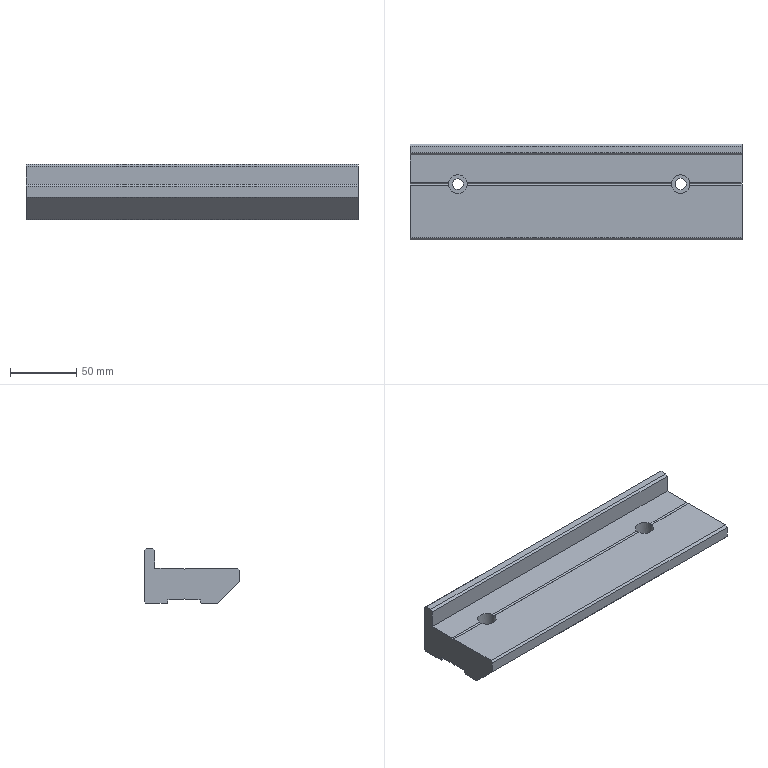Part | NX | features EXTRUDE 3, DATUM_CSYS 2, SKETCH 1 | 1 solid | 39 faces | box 250 x 72 x 41.5 mm | volume 446626 mm3 | plane 35 | cylinder 4 | commonest cylinder face diameters 14 x2 8 x1 8.5 x1
STEP:
#1=CARTESIAN_POINT('',(4843.54,6881.489,-37.5));
#2=VERTEX_POINT('',#1);
#3=CARTESIAN_POINT('',(4843.413,6882.489,-38.5));
#4=VERTEX_POINT('',#3);
#5=CARTESIAN_POINT('',(4839.54,6881.489,-37.5));
#6=DIRECTION('',(0.,-0.7071,-0.7071));
#7=DIRECTION('',(0.,-0.7071,0.7071));
#8=AXIS2_PLACEMENT_3D('',#5,#6,#7);
#9=ELLIPSE('',#8,5.657,4.);
#10=EDGE_CURVE('',#2,#4,#9,.F.);
#11=ORIENTED_EDGE('',*,*,#10,.F.);
#12=CARTESIAN_POINT('',(4843.413,6880.489,-38.5));
#13=VERTEX_POINT('',#12);
#14=CARTESIAN_POINT('',(4839.54,6881.489,-37.5));
#15=DIRECTION('',(0.,0.7071,-0.7071));
#16=DIRECTION('',(0.,0.7071,0.7071));
#17=AXIS2_PLACEMENT_3D('',#14,#15,#16);
#18=ELLIPSE('',#17,5.657,4.);
#19=EDGE_CURVE('',#13,#2,#18,.F.);
#20=ORIENTED_EDGE('',*,*,#19,.F.);
#21=CARTESIAN_POINT('',(4835.667,6880.489,-38.5));
#22=VERTEX_POINT('',#21);
#23=CARTESIAN_POINT('',(4839.54,6881.489,-38.5));
#24=DIRECTION('',(0.,0.,-1.));
#25=DIRECTION('',(-1.,0.,0.));
#26=AXIS2_PLACEMENT_3D('',#23,#24,#25);
#27=CIRCLE('',#26,4.);
#28=EDGE_CURVE('',#22,#13,#27,.F.);
#29=ORIENTED_EDGE('',*,*,#28,.F.);
#30=CARTESIAN_POINT('',(4835.54,6881.489,-37.5));
#31=VERTEX_POINT('',#30);
#32=CARTESIAN_POINT('',(4839.54,6881.489,-37.5));
#33=DIRECTION('',(0.,0.7071,-0.7071));
#34=DIRECTION('',(0.,0.7071,0.7071));
#35=AXIS2_PLACEMENT_3D('',#32,#33,#34);
#36=ELLIPSE('',#35,5.657,4.);
#37=EDGE_CURVE('',#31,#22,#36,.F.);
#38=ORIENTED_EDGE('',*,*,#37,.F.);
#39=CARTESIAN_POINT('',(4835.667,6882.489,-38.5));
#40=VERTEX_POINT('',#39);
#41=CARTESIAN_POINT('',(4839.54,6881.489,-37.5));
#42=DIRECTION('',(0.,-0.7071,-0.7071));
#43=DIRECTION('',(0.,-0.7071,0.7071));
#44=AXIS2_PLACEMENT_3D('',#41,#42,#43);
#45=ELLIPSE('',#44,5.657,4.);
#46=EDGE_CURVE('',#40,#31,#45,.F.);
#47=ORIENTED_EDGE('',*,*,#46,.F.);
#48=CARTESIAN_POINT('',(4839.54,6881.489,-38.5));
#49=DIRECTION('',(0.,0.,-1.));
#50=DIRECTION('',(-1.,0.,0.));
#51=AXIS2_PLACEMENT_3D('',#48,#49,#50);
#52=CIRCLE('',#51,4.);
#53=EDGE_CURVE('',#4,#40,#52,.F.);
#54=ORIENTED_EDGE('',*,*,#53,.F.);
#55=EDGE_LOOP('',(#11,#20,#29,#38,#47,#54));
#56=FACE_BOUND('',#55,.T.);
#57=CARTESIAN_POINT('',(4843.54,6881.489,-27.));
#58=VERTEX_POINT('',#57);
#59=CARTESIAN_POINT('',(4839.54,6881.489,-27.));
#60=DIRECTION('',(0.,0.,1.));
#61=DIRECTION('',(1.,0.,0.));
#62=AXIS2_PLACEMENT_3D('',#59,#60,#61);
#63=CIRCLE('',#62,4.);
#64=EDGE_CURVE('',#58,#58,#63,.F.);
#65=ORIENTED_EDGE('',*,*,#64,.F.);
#66=EDGE_LOOP('',(#65));
#67=FACE_BOUND('',#66,.T.);
#68=CARTESIAN_POINT('',(4839.54,6881.489,-55015.));
#69=DIRECTION('',(0.,0.,1.));
#70=DIRECTION('',(1.,0.,0.));
#71=AXIS2_PLACEMENT_3D('',#68,#69,#70);
#72=CYLINDRICAL_SURFACE('',#71,4.);
#73=ADVANCED_FACE('',(#56,#67),#72,.F.);
#74=CARTESIAN_POINT('',(5011.563,6881.489,-37.5));
#75=VERTEX_POINT('',#74);
#76=CARTESIAN_POINT('',(5011.444,6882.489,-38.5));
#77=VERTEX_POINT('',#76);
#78=CARTESIAN_POINT('',(5007.313,6881.489,-37.5));
#79=DIRECTION('',(0.,-0.7071,-0.7071));
#80=DIRECTION('',(0.,-0.7071,0.7071));
#81=AXIS2_PLACEMENT_3D('',#78,#79,#80);
#82=ELLIPSE('',#81,6.01,4.25);
#83=EDGE_CURVE('',#75,#77,#82,.F.);
#84=ORIENTED_EDGE('',*,*,#83,.F.);
#85=CARTESIAN_POINT('',(5011.444,6880.489,-38.5));
#86=VERTEX_POINT('',#85);
#87=CARTESIAN_POINT('',(5007.313,6881.489,-37.5));
#88=DIRECTION('',(0.,0.7071,-0.7071));
#89=DIRECTION('',(0.,0.7071,0.7071));
#90=AXIS2_PLACEMENT_3D('',#87,#88,#89);
#91=ELLIPSE('',#90,6.01,4.25);
#92=EDGE_CURVE('',#86,#75,#91,.F.);
#93=ORIENTED_EDGE('',*,*,#92,.F.);
#94=CARTESIAN_POINT('',(5003.182,6880.489,-38.5));
#95=VERTEX_POINT('',#94);
#96=CARTESIAN_POINT('',(5007.313,6881.489,-38.5));
#97=DIRECTION('',(0.,0.,-1.));
#98=DIRECTION('',(-1.,0.,0.));
#99=AXIS2_PLACEMENT_3D('',#96,#97,#98);
#100=CIRCLE('',#99,4.25);
#101=EDGE_CURVE('',#95,#86,#100,.F.);
#102=ORIENTED_EDGE('',*,*,#101,.F.);
#103=CARTESIAN_POINT('',(5003.063,6881.489,-37.5));
#104=VERTEX_POINT('',#103);
#105=CARTESIAN_POINT('',(5007.313,6881.489,-37.5));
#106=DIRECTION('',(0.,0.7071,-0.7071));
#107=DIRECTION('',(0.,0.7071,0.7071));
#108=AXIS2_PLACEMENT_3D('',#105,#106,#107);
#109=ELLIPSE('',#108,6.01,4.25);
#110=EDGE_CURVE('',#104,#95,#109,.F.);
#111=ORIENTED_EDGE('',*,*,#110,.F.);
#112=CARTESIAN_POINT('',(5003.182,6882.489,-38.5));
#113=VERTEX_POINT('',#112);
#114=CARTESIAN_POINT('',(5007.313,6881.489,-37.5));
#115=DIRECTION('',(0.,-0.7071,-0.7071));
#116=DIRECTION('',(0.,-0.7071,0.7071));
#117=AXIS2_PLACEMENT_3D('',#114,#115,#116);
#118=ELLIPSE('',#117,6.01,4.25);
#119=EDGE_CURVE('',#113,#104,#118,.F.);
#120=ORIENTED_EDGE('',*,*,#119,.F.);
#121=CARTESIAN_POINT('',(5007.313,6881.489,-38.5));
#122=DIRECTION('',(0.,0.,-1.));
#123=DIRECTION('',(-1.,0.,0.));
#124=AXIS2_PLACEMENT_3D('',#121,#122,#123);
#125=CIRCLE('',#124,4.25);
#126=EDGE_CURVE('',#77,#113,#125,.F.);
#127=ORIENTED_EDGE('',*,*,#126,.F.);
#128=EDGE_LOOP('',(#84,#93,#102,#111,#120,#127));
#129=FACE_BOUND('',#128,.T.);
#130=CARTESIAN_POINT('',(5011.563,6881.489,-27.));
#131=VERTEX_POINT('',#130);
#132=CARTESIAN_POINT('',(5007.313,6881.489,-27.));
#133=DIRECTION('',(0.,0.,1.));
#134=DIRECTION('',(1.,0.,0.));
#135=AXIS2_PLACEMENT_3D('',#132,#133,#134);
#136=CIRCLE('',#135,4.25);
#137=EDGE_CURVE('',#131,#131,#136,.F.);
#138=ORIENTED_EDGE('',*,*,#137,.F.);
#139=EDGE_LOOP('',(#138));
#140=FACE_BOUND('',#139,.T.);
#141=CARTESIAN_POINT('',(5007.313,6881.489,-55015.));
#142=DIRECTION('',(0.,0.,1.));
#143=DIRECTION('',(1.,0.,0.));
#144=AXIS2_PLACEMENT_3D('',#141,#142,#143);
#145=CYLINDRICAL_SURFACE('',#144,4.25);
#146=ADVANCED_FACE('',(#129,#140),#145,.F.);
#147=CARTESIAN_POINT('',(5000.385,6882.489,-15.));
#148=VERTEX_POINT('',#147);
#149=CARTESIAN_POINT('',(5000.313,6881.489,-16.));
#150=VERTEX_POINT('',#149);
#151=CARTESIAN_POINT('',(5007.313,6881.489,-16.));
#152=DIRECTION('',(0.,-0.7071,0.7071));
#153=DIRECTION('',(0.,0.7071,0.7071));
#154=AXIS2_PLACEMENT_3D('',#151,#152,#153);
#155=ELLIPSE('',#154,9.899,7.);
#156=EDGE_CURVE('',#148,#150,#155,.T.);
#157=ORIENTED_EDGE('',*,*,#156,.F.);
#158=CARTESIAN_POINT('',(4846.468,6882.489,-15.));
#159=VERTEX_POINT('',#158);
#160=CARTESIAN_POINT('',(4803.499,6882.489,-15.));
#161=DIRECTION('',(1.,0.,0.));
#162=VECTOR('',#161,1000.);
#163=LINE('',#160,#162);
#164=EDGE_CURVE('',#159,#148,#163,.T.);
#165=ORIENTED_EDGE('',*,*,#164,.F.);
#166=CARTESIAN_POINT('',(4846.54,6881.489,-16.));
#167=VERTEX_POINT('',#166);
#168=CARTESIAN_POINT('',(4839.54,6881.489,-16.));
#169=DIRECTION('',(0.,-0.7071,0.7071));
#170=DIRECTION('',(0.,0.7071,0.7071));
#171=AXIS2_PLACEMENT_3D('',#168,#169,#170);
#172=ELLIPSE('',#171,9.899,7.);
#173=EDGE_CURVE('',#167,#159,#172,.T.);
#174=ORIENTED_EDGE('',*,*,#173,.F.);
#175=CARTESIAN_POINT('',(4803.499,6881.489,-16.));
#176=DIRECTION('',(1.,0.,0.));
#177=VECTOR('',#176,1000.);
#178=LINE('',#175,#177);
#179=EDGE_CURVE('',#167,#150,#178,.T.);
#180=ORIENTED_EDGE('',*,*,#179,.T.);
#181=EDGE_LOOP('',(#157,#165,#174,#180));
#182=FACE_BOUND('',#181,.T.);
#183=CARTESIAN_POINT('',(4803.499,6882.489,-15.));
#184=DIRECTION('',(0.,-0.7071,0.7071));
#185=DIRECTION('',(0.,-0.7071,-0.7071));
#186=AXIS2_PLACEMENT_3D('',#183,#184,#185);
#187=PLANE('',#186);
#188=ADVANCED_FACE('',(#182),#187,.T.);
#189=CARTESIAN_POINT('',(4832.612,6882.489,-15.));
#190=VERTEX_POINT('',#189);
#191=CARTESIAN_POINT('',(4832.54,6881.489,-16.));
#192=VERTEX_POINT('',#191);
#193=CARTESIAN_POINT('',(4839.54,6881.489,-16.));
#194=DIRECTION('',(0.,-0.7071,0.7071));
#195=DIRECTION('',(0.,0.7071,0.7071));
#196=AXIS2_PLACEMENT_3D('',#193,#194,#195);
#197=ELLIPSE('',#196,9.899,7.);
#198=EDGE_CURVE('',#190,#192,#197,.T.);
#199=ORIENTED_EDGE('',*,*,#198,.F.);
#200=CARTESIAN_POINT('',(4803.499,6882.489,-15.));
#201=VERTEX_POINT('',#200);
#202=CARTESIAN_POINT('',(4803.499,6882.489,-15.));
#203=DIRECTION('',(1.,0.,0.));
#204=VECTOR('',#203,1000.);
#205=LINE('',#202,#204);
#206=EDGE_CURVE('',#201,#190,#205,.T.);
#207=ORIENTED_EDGE('',*,*,#206,.F.);
#208=CARTESIAN_POINT('',(4803.499,6881.489,-16.));
#209=VERTEX_POINT('',#208);
#210=CARTESIAN_POINT('',(4803.499,6882.489,-15.));
#211=DIRECTION('',(0.,-0.7071,-0.7071));
#212=VECTOR('',#211,1000.);
#213=LINE('',#210,#212);
#214=EDGE_CURVE('',#201,#209,#213,.T.);
#215=ORIENTED_EDGE('',*,*,#214,.T.);
#216=CARTESIAN_POINT('',(4803.499,6881.489,-16.));
#217=DIRECTION('',(1.,0.,0.));
#218=VECTOR('',#217,1000.);
#219=LINE('',#216,#218);
#220=EDGE_CURVE('',#209,#192,#219,.T.);
#221=ORIENTED_EDGE('',*,*,#220,.T.);
#222=EDGE_LOOP('',(#199,#207,#215,#221));
#223=FACE_BOUND('',#222,.T.);
#224=CARTESIAN_POINT('',(4803.499,6882.489,-15.));
#225=DIRECTION('',(0.,-0.7071,0.7071));
#226=DIRECTION('',(0.,-0.7071,-0.7071));
#227=AXIS2_PLACEMENT_3D('',#224,#225,#226);
#228=PLANE('',#227);
#229=ADVANCED_FACE('',(#223),#228,.T.);
#230=CARTESIAN_POINT('',(5014.241,6880.489,-15.));
#231=VERTEX_POINT('',#230);
#232=CARTESIAN_POINT('',(5014.313,6881.489,-16.));
#233=VERTEX_POINT('',#232);
#234=CARTESIAN_POINT('',(5007.313,6881.489,-16.));
#235=DIRECTION('',(0.,0.7071,0.7071));
#236=DIRECTION('',(0.,-0.7071,0.7071));
#237=AXIS2_PLACEMENT_3D('',#234,#235,#236);
#238=ELLIPSE('',#237,9.899,7.);
#239=EDGE_CURVE('',#231,#233,#238,.T.);
#240=ORIENTED_EDGE('',*,*,#239,.F.);
#241=CARTESIAN_POINT('',(5053.499,6880.489,-15.));
#242=VERTEX_POINT('',#241);
#243=CARTESIAN_POINT('',(4803.499,6880.489,-15.));
#244=DIRECTION('',(1.,0.,0.));
#245=VECTOR('',#244,1000.);
#246=LINE('',#243,#245);
#247=EDGE_CURVE('',#231,#242,#246,.T.);
#248=ORIENTED_EDGE('',*,*,#247,.T.);
#249=CARTESIAN_POINT('',(5053.499,6881.489,-16.));
#250=VERTEX_POINT('',#249);
#251=CARTESIAN_POINT('',(5053.499,6881.489,-16.));
#252=DIRECTION('',(0.,-0.7071,0.7071));
#253=VECTOR('',#252,1000.);
#254=LINE('',#251,#253);
#255=EDGE_CURVE('',#250,#242,#254,.T.);
#256=ORIENTED_EDGE('',*,*,#255,.F.);
#257=CARTESIAN_POINT('',(4803.499,6881.489,-16.));
#258=DIRECTION('',(1.,0.,0.));
#259=VECTOR('',#258,1000.);
#260=LINE('',#257,#259);
#261=EDGE_CURVE('',#233,#250,#260,.T.);
#262=ORIENTED_EDGE('',*,*,#261,.F.);
#263=EDGE_LOOP('',(#240,#248,#256,#262));
#264=FACE_BOUND('',#263,.T.);
#265=CARTESIAN_POINT('',(4803.499,6881.489,-16.));
#266=DIRECTION('',(0.,0.7071,0.7071));
#267=DIRECTION('',(0.,-0.7071,0.7071));
#268=AXIS2_PLACEMENT_3D('',#265,#266,#267);
#269=PLANE('',#268);
#270=ADVANCED_FACE('',(#264),#269,.T.);
#271=CARTESIAN_POINT('',(5000.385,6880.489,-15.));
#272=VERTEX_POINT('',#271);
#273=CARTESIAN_POINT('',(5007.313,6881.489,-16.));
#274=DIRECTION('',(0.,0.7071,0.7071));
#275=DIRECTION('',(0.,-0.7071,0.7071));
#276=AXIS2_PLACEMENT_3D('',#273,#274,#275);
#277=ELLIPSE('',#276,9.899,7.);
#278=EDGE_CURVE('',#150,#272,#277,.T.);
#279=ORIENTED_EDGE('',*,*,#278,.F.);
#280=ORIENTED_EDGE('',*,*,#179,.F.);
#281=CARTESIAN_POINT('',(4846.468,6880.489,-15.));
#282=VERTEX_POINT('',#281);
#283=CARTESIAN_POINT('',(4839.54,6881.489,-16.));
#284=DIRECTION('',(0.,0.7071,0.7071));
#285=DIRECTION('',(0.,-0.7071,0.7071));
#286=AXIS2_PLACEMENT_3D('',#283,#284,#285);
#287=ELLIPSE('',#286,9.899,7.);
#288=EDGE_CURVE('',#282,#167,#287,.T.);
#289=ORIENTED_EDGE('',*,*,#288,.F.);
#290=CARTESIAN_POINT('',(4803.499,6880.489,-15.));
#291=DIRECTION('',(1.,0.,0.));
#292=VECTOR('',#291,1000.);
#293=LINE('',#290,#292);
#294=EDGE_CURVE('',#282,#272,#293,.T.);
#295=ORIENTED_EDGE('',*,*,#294,.T.);
#296=EDGE_LOOP('',(#279,#280,#289,#295));
#297=FACE_BOUND('',#296,.T.);
#298=CARTESIAN_POINT('',(4803.499,6881.489,-16.));
#299=DIRECTION('',(0.,0.7071,0.7071));
#300=DIRECTION('',(0.,-0.7071,0.7071));
#301=AXIS2_PLACEMENT_3D('',#298,#299,#300);
#302=PLANE('',#301);
#303=ADVANCED_FACE('',(#297),#302,.T.);
#304=CARTESIAN_POINT('',(4803.499,6880.489,-38.5));
#305=DIRECTION('',(1.,0.,0.));
#306=VECTOR('',#305,1000.);
#307=LINE('',#304,#306);
#308=EDGE_CURVE('',#13,#95,#307,.T.);
#309=ORIENTED_EDGE('',*,*,#308,.T.);
#310=ORIENTED_EDGE('',*,*,#101,.T.);
#311=CARTESIAN_POINT('',(5053.499,6880.489,-38.5));
#312=VERTEX_POINT('',#311);
#313=CARTESIAN_POINT('',(4803.499,6880.489,-38.5));
#314=DIRECTION('',(1.,0.,0.));
#315=VECTOR('',#314,1000.);
#316=LINE('',#313,#315);
#317=EDGE_CURVE('',#86,#312,#316,.T.);
#318=ORIENTED_EDGE('',*,*,#317,.T.);
#319=CARTESIAN_POINT('',(5053.499,6869.414,-38.5));
#320=VERTEX_POINT('',#319);
#321=CARTESIAN_POINT('',(5053.499,6869.414,-38.5));
#322=DIRECTION('',(0.,1.,0.));
#323=VECTOR('',#322,1000.);
#324=LINE('',#321,#323);
#325=EDGE_CURVE('',#320,#312,#324,.T.);
#326=ORIENTED_EDGE('',*,*,#325,.F.);
#327=CARTESIAN_POINT('',(4803.499,6869.414,-38.5));
#328=VERTEX_POINT('',#327);
#329=CARTESIAN_POINT('',(4803.499,6869.414,-38.5));
#330=DIRECTION('',(1.,0.,0.));
#331=VECTOR('',#330,1000.);
#332=LINE('',#329,#331);
#333=EDGE_CURVE('',#328,#320,#332,.T.);
#334=ORIENTED_EDGE('',*,*,#333,.F.);
#335=CARTESIAN_POINT('',(4803.499,6880.489,-38.5));
#336=VERTEX_POINT('',#335);
#337=CARTESIAN_POINT('',(4803.499,6869.414,-38.5));
#338=DIRECTION('',(0.,1.,0.));
#339=VECTOR('',#338,1000.);
#340=LINE('',#337,#339);
#341=EDGE_CURVE('',#328,#336,#340,.T.);
#342=ORIENTED_EDGE('',*,*,#341,.T.);
#343=CARTESIAN_POINT('',(4803.499,6880.489,-38.5));
#344=DIRECTION('',(1.,0.,0.));
#345=VECTOR('',#344,1000.);
#346=LINE('',#343,#345);
#347=EDGE_CURVE('',#336,#22,#346,.T.);
#348=ORIENTED_EDGE('',*,*,#347,.T.);
#349=ORIENTED_EDGE('',*,*,#28,.T.);
#350=EDGE_LOOP('',(#309,#310,#318,#326,#334,#342,#348,#349));
#351=FACE_BOUND('',#350,.T.);
#352=CARTESIAN_POINT('',(4803.499,6869.414,-38.5));
#353=DIRECTION('',(0.,0.,-1.));
#354=DIRECTION('',(-1.,0.,0.));
#355=AXIS2_PLACEMENT_3D('',#352,#353,#354);
#356=PLANE('',#355);
#357=ADVANCED_FACE('',(#351),#356,.T.);
#358=CARTESIAN_POINT('',(4803.499,6881.489,-37.5));
#359=DIRECTION('',(1.,0.,0.));
#360=VECTOR('',#359,1000.);
#361=LINE('',#358,#360);
#362=EDGE_CURVE('',#2,#104,#361,.T.);
#363=ORIENTED_EDGE('',*,*,#362,.T.);
#364=ORIENTED_EDGE('',*,*,#110,.T.);
#365=ORIENTED_EDGE('',*,*,#308,.F.);
#366=ORIENTED_EDGE('',*,*,#19,.T.);
#367=EDGE_LOOP('',(#363,#364,#365,#366));
#368=FACE_BOUND('',#367,.T.);
#369=CARTESIAN_POINT('',(4803.499,6880.489,-38.5));
#370=DIRECTION('',(0.,0.7071,-0.7071));
#371=DIRECTION('',(0.,0.7071,0.7071));
#372=AXIS2_PLACEMENT_3D('',#369,#370,#371);
#373=PLANE('',#372);
#374=ADVANCED_FACE('',(#368),#373,.T.);
#375=ORIENTED_EDGE('',*,*,#317,.F.);
#376=ORIENTED_EDGE('',*,*,#92,.T.);
#377=CARTESIAN_POINT('',(5053.499,6881.489,-37.5));
#378=VERTEX_POINT('',#377);
#379=CARTESIAN_POINT('',(4803.499,6881.489,-37.5));
#380=DIRECTION('',(1.,0.,0.));
#381=VECTOR('',#380,1000.);
#382=LINE('',#379,#381);
#383=EDGE_CURVE('',#75,#378,#382,.T.);
#384=ORIENTED_EDGE('',*,*,#383,.T.);
#385=CARTESIAN_POINT('',(5053.499,6880.489,-38.5));
#386=DIRECTION('',(0.,0.7071,0.7071));
#387=VECTOR('',#386,1000.);
#388=LINE('',#385,#387);
#389=EDGE_CURVE('',#312,#378,#388,.T.);
#390=ORIENTED_EDGE('',*,*,#389,.F.);
#391=EDGE_LOOP('',(#375,#376,#384,#390));
#392=FACE_BOUND('',#391,.T.);
#393=CARTESIAN_POINT('',(4803.499,6880.489,-38.5));
#394=DIRECTION('',(0.,0.7071,-0.7071));
#395=DIRECTION('',(0.,0.7071,0.7071));
#396=AXIS2_PLACEMENT_3D('',#393,#394,#395);
#397=PLANE('',#396);
#398=ADVANCED_FACE('',(#392),#397,.T.);
#399=CARTESIAN_POINT('',(4803.499,6881.489,-37.5));
#400=VERTEX_POINT('',#399);
#401=CARTESIAN_POINT('',(4803.499,6881.489,-37.5));
#402=DIRECTION('',(1.,0.,0.));
#403=VECTOR('',#402,1000.);
#404=LINE('',#401,#403);
#405=EDGE_CURVE('',#400,#31,#404,.T.);
#406=ORIENTED_EDGE('',*,*,#405,.T.);
#407=ORIENTED_EDGE('',*,*,#37,.T.);
#408=ORIENTED_EDGE('',*,*,#347,.F.);
#409=CARTESIAN_POINT('',(4803.499,6880.489,-38.5));
#410=DIRECTION('',(0.,0.7071,0.7071));
#411=VECTOR('',#410,1000.);
#412=LINE('',#409,#411);
#413=EDGE_CURVE('',#336,#400,#412,.T.);
#414=ORIENTED_EDGE('',*,*,#413,.T.);
#415=EDGE_LOOP('',(#406,#407,#408,#414));
#416=FACE_BOUND('',#415,.T.);
#417=CARTESIAN_POINT('',(4803.499,6880.489,-38.5));
#418=DIRECTION('',(0.,0.7071,-0.7071));
#419=DIRECTION('',(0.,0.7071,0.7071));
#420=AXIS2_PLACEMENT_3D('',#417,#418,#419);
#421=PLANE('',#420);
#422=ADVANCED_FACE('',(#416),#421,.T.);
#423=ORIENTED_EDGE('',*,*,#383,.F.);
#424=ORIENTED_EDGE('',*,*,#83,.T.);
#425=CARTESIAN_POINT('',(5053.499,6882.489,-38.5));
#426=VERTEX_POINT('',#425);
#427=CARTESIAN_POINT('',(4803.499,6882.489,-38.5));
#428=DIRECTION('',(1.,0.,0.));
#429=VECTOR('',#428,1000.);
#430=LINE('',#427,#429);
#431=EDGE_CURVE('',#77,#426,#430,.T.);
#432=ORIENTED_EDGE('',*,*,#431,.T.);
#433=CARTESIAN_POINT('',(5053.499,6881.489,-37.5));
#434=DIRECTION('',(0.,0.7071,-0.7071));
#435=VECTOR('',#434,1000.);
#436=LINE('',#433,#435);
#437=EDGE_CURVE('',#378,#426,#436,.T.);
#438=ORIENTED_EDGE('',*,*,#437,.F.);
#439=EDGE_LOOP('',(#423,#424,#432,#438));
#440=FACE_BOUND('',#439,.T.);
#441=CARTESIAN_POINT('',(4803.499,6881.489,-37.5));
#442=DIRECTION('',(0.,-0.7071,-0.7071));
#443=DIRECTION('',(0.,0.7071,-0.7071));
#444=AXIS2_PLACEMENT_3D('',#441,#442,#443);
#445=PLANE('',#444);
#446=ADVANCED_FACE('',(#440),#445,.T.);
#447=CARTESIAN_POINT('',(4803.499,6882.489,-38.5));
#448=DIRECTION('',(1.,0.,0.));
#449=VECTOR('',#448,1000.);
#450=LINE('',#447,#449);
#451=EDGE_CURVE('',#4,#113,#450,.T.);
#452=ORIENTED_EDGE('',*,*,#451,.T.);
#453=ORIENTED_EDGE('',*,*,#119,.T.);
#454=ORIENTED_EDGE('',*,*,#362,.F.);
#455=ORIENTED_EDGE('',*,*,#10,.T.);
#456=EDGE_LOOP('',(#452,#453,#454,#455));
#457=FACE_BOUND('',#456,.T.);
#458=CARTESIAN_POINT('',(4803.499,6881.489,-37.5));
#459=DIRECTION('',(0.,-0.7071,-0.7071));
#460=DIRECTION('',(0.,0.7071,-0.7071));
#461=AXIS2_PLACEMENT_3D('',#458,#459,#460);
#462=PLANE('',#461);
#463=ADVANCED_FACE('',(#457),#462,.T.);
#464=CARTESIAN_POINT('',(4803.499,6882.489,-38.5));
#465=VERTEX_POINT('',#464);
#466=CARTESIAN_POINT('',(4803.499,6882.489,-38.5));
#467=DIRECTION('',(1.,0.,0.));
#468=VECTOR('',#467,1000.);
#469=LINE('',#466,#468);
#470=EDGE_CURVE('',#465,#40,#469,.T.);
#471=ORIENTED_EDGE('',*,*,#470,.T.);
#472=ORIENTED_EDGE('',*,*,#46,.T.);
#473=ORIENTED_EDGE('',*,*,#405,.F.);
#474=CARTESIAN_POINT('',(4803.499,6881.489,-37.5));
#475=DIRECTION('',(0.,0.7071,-0.7071));
#476=VECTOR('',#475,1000.);
#477=LINE('',#474,#476);
#478=EDGE_CURVE('',#400,#465,#477,.T.);
#479=ORIENTED_EDGE('',*,*,#478,.T.);
#480=EDGE_LOOP('',(#471,#472,#473,#479));
#481=FACE_BOUND('',#480,.T.);
#482=CARTESIAN_POINT('',(4803.499,6881.489,-37.5));
#483=DIRECTION('',(0.,-0.7071,-0.7071));
#484=DIRECTION('',(0.,0.7071,-0.7071));
#485=AXIS2_PLACEMENT_3D('',#482,#483,#484);
#486=PLANE('',#485);
#487=ADVANCED_FACE('',(#481),#486,.T.);
#488=ORIENTED_EDGE('',*,*,#431,.F.);
#489=ORIENTED_EDGE('',*,*,#126,.T.);
#490=ORIENTED_EDGE('',*,*,#451,.F.);
#491=ORIENTED_EDGE('',*,*,#53,.T.);
#492=ORIENTED_EDGE('',*,*,#470,.F.);
#493=CARTESIAN_POINT('',(4803.499,6893.564,-38.5));
#494=VERTEX_POINT('',#493);
#495=CARTESIAN_POINT('',(4803.499,6882.489,-38.5));
#496=DIRECTION('',(0.,1.,0.));
#497=VECTOR('',#496,1000.);
#498=LINE('',#495,#497);
#499=EDGE_CURVE('',#465,#494,#498,.T.);
#500=ORIENTED_EDGE('',*,*,#499,.T.);
#501=CARTESIAN_POINT('',(5053.499,6893.564,-38.5));
#502=VERTEX_POINT('',#501);
#503=CARTESIAN_POINT('',(4803.499,6893.564,-38.5));
#504=DIRECTION('',(1.,0.,0.));
#505=VECTOR('',#504,1000.);
#506=LINE('',#503,#505);
#507=EDGE_CURVE('',#494,#502,#506,.T.);
#508=ORIENTED_EDGE('',*,*,#507,.T.);
#509=CARTESIAN_POINT('',(5053.499,6882.489,-38.5));
#510=DIRECTION('',(0.,1.,0.));
#511=VECTOR('',#510,1000.);
#512=LINE('',#509,#511);
#513=EDGE_CURVE('',#426,#502,#512,.T.);
#514=ORIENTED_EDGE('',*,*,#513,.F.);
#515=EDGE_LOOP('',(#488,#489,#490,#491,#492,#500,#508,#514));
#516=FACE_BOUND('',#515,.T.);
#517=CARTESIAN_POINT('',(4803.499,6882.489,-38.5));
#518=DIRECTION('',(0.,0.,-1.));
#519=DIRECTION('',(-1.,0.,0.));
#520=AXIS2_PLACEMENT_3D('',#517,#518,#519);
#521=PLANE('',#520);
#522=ADVANCED_FACE('',(#516),#521,.T.);
#523=CARTESIAN_POINT('',(5053.499,6911.489,-40.3));
#524=VERTEX_POINT('',#523);
#525=CARTESIAN_POINT('',(5053.499,6911.489,-1.5));
#526=VERTEX_POINT('',#525);
#527=CARTESIAN_POINT('',(5053.499,6911.489,-40.3));
#528=DIRECTION('',(0.,0.,1.));
#529=VECTOR('',#528,1000.);
#530=LINE('',#527,#529);
#531=EDGE_CURVE('',#524,#526,#530,.T.);
#532=ORIENTED_EDGE('',*,*,#531,.F.);
#533=CARTESIAN_POINT('',(4803.499,6911.489,-40.3));
#534=VERTEX_POINT('',#533);
#535=CARTESIAN_POINT('',(4803.499,6911.489,-40.3));
#536=DIRECTION('',(1.,0.,0.));
#537=VECTOR('',#536,1000.);
#538=LINE('',#535,#537);
#539=EDGE_CURVE('',#534,#524,#538,.T.);
#540=ORIENTED_EDGE('',*,*,#539,.F.);
#541=CARTESIAN_POINT('',(4803.499,6911.489,-1.5));
#542=VERTEX_POINT('',#541);
#543=CARTESIAN_POINT('',(4803.499,6911.489,-40.3));
#544=DIRECTION('',(0.,0.,1.));
#545=VECTOR('',#544,1000.);
#546=LINE('',#543,#545);
#547=EDGE_CURVE('',#534,#542,#546,.T.);
#548=ORIENTED_EDGE('',*,*,#547,.T.);
#549=CARTESIAN_POINT('',(4803.499,6911.489,-1.5));
#550=DIRECTION('',(1.,0.,0.));
#551=VECTOR('',#550,1000.);
#552=LINE('',#549,#551);
#553=EDGE_CURVE('',#542,#526,#552,.T.);
#554=ORIENTED_EDGE('',*,*,#553,.T.);
#555=EDGE_LOOP('',(#532,#540,#548,#554));
#556=FACE_BOUND('',#555,.T.);
#557=CARTESIAN_POINT('',(4803.499,6911.489,-40.3));
#558=DIRECTION('',(0.,1.,0.));
#559=DIRECTION('',(0.,0.,1.));
#560=AXIS2_PLACEMENT_3D('',#557,#558,#559);
#561=PLANE('',#560);
#562=ADVANCED_FACE('',(#556),#561,.T.);
#563=CARTESIAN_POINT('',(5053.499,6909.989,0.));
#564=VERTEX_POINT('',#563);
#565=CARTESIAN_POINT('',(5053.499,6911.489,-1.5));
#566=DIRECTION('',(0.,-0.7071,0.7071));
#567=VECTOR('',#566,1000.);
#568=LINE('',#565,#567);
#569=EDGE_CURVE('',#526,#564,#568,.T.);
#570=ORIENTED_EDGE('',*,*,#569,.F.);
#571=ORIENTED_EDGE('',*,*,#553,.F.);
#572=CARTESIAN_POINT('',(4803.499,6909.989,0.));
#573=VERTEX_POINT('',#572);
#574=CARTESIAN_POINT('',(4803.499,6911.489,-1.5));
#575=DIRECTION('',(0.,-0.7071,0.7071));
#576=VECTOR('',#575,1000.);
#577=LINE('',#574,#576);
#578=EDGE_CURVE('',#542,#573,#577,.T.);
#579=ORIENTED_EDGE('',*,*,#578,.T.);
#580=CARTESIAN_POINT('',(4803.499,6909.989,0.));
#581=DIRECTION('',(1.,0.,0.));
#582=VECTOR('',#581,1000.);
#583=LINE('',#580,#582);
#584=EDGE_CURVE('',#573,#564,#583,.T.);
#585=ORIENTED_EDGE('',*,*,#584,.T.);
#586=EDGE_LOOP('',(#570,#571,#579,#585));
#587=FACE_BOUND('',#586,.T.);
#588=CARTESIAN_POINT('',(4803.499,6911.489,-1.5));
#589=DIRECTION('',(0.,0.7071,0.7071));
#590=DIRECTION('',(0.,-0.7071,0.7071));
#591=AXIS2_PLACEMENT_3D('',#588,#589,#590);
#592=PLANE('',#591);
#593=ADVANCED_FACE('',(#587),#592,.T.);
#594=CARTESIAN_POINT('',(5053.499,6904.989,0.));
#595=VERTEX_POINT('',#594);
#596=CARTESIAN_POINT('',(5053.499,6909.989,0.));
#597=DIRECTION('',(0.,-1.,0.));
#598=VECTOR('',#597,1000.);
#599=LINE('',#596,#598);
#600=EDGE_CURVE('',#564,#595,#599,.T.);
#601=ORIENTED_EDGE('',*,*,#600,.F.);
#602=ORIENTED_EDGE('',*,*,#584,.F.);
#603=CARTESIAN_POINT('',(4803.499,6904.989,0.));
#604=VERTEX_POINT('',#603);
#605=CARTESIAN_POINT('',(4803.499,6909.989,0.));
#606=DIRECTION('',(0.,-1.,0.));
#607=VECTOR('',#606,1000.);
#608=LINE('',#605,#607);
#609=EDGE_CURVE('',#573,#604,#608,.T.);
#610=ORIENTED_EDGE('',*,*,#609,.T.);
#611=CARTESIAN_POINT('',(4803.499,6904.989,0.));
#612=DIRECTION('',(1.,0.,0.));
#613=VECTOR('',#612,1000.);
#614=LINE('',#611,#613);
#615=EDGE_CURVE('',#604,#595,#614,.T.);
#616=ORIENTED_EDGE('',*,*,#615,.T.);
#617=EDGE_LOOP('',(#601,#602,#610,#616));
#618=FACE_BOUND('',#617,.T.);
#619=CARTESIAN_POINT('',(4803.499,6909.989,0.));
#620=DIRECTION('',(0.,0.,1.));
#621=DIRECTION('',(1.,0.,0.));
#622=AXIS2_PLACEMENT_3D('',#619,#620,#621);
#623=PLANE('',#622);
#624=ADVANCED_FACE('',(#618),#623,.T.);
#625=CARTESIAN_POINT('',(5053.499,6903.489,-1.5));
#626=VERTEX_POINT('',#625);
#627=CARTESIAN_POINT('',(5053.499,6904.989,0.));
#628=DIRECTION('',(0.,-0.7071,-0.7071));
#629=VECTOR('',#628,1000.);
#630=LINE('',#627,#629);
#631=EDGE_CURVE('',#595,#626,#630,.T.);
#632=ORIENTED_EDGE('',*,*,#631,.F.);
#633=ORIENTED_EDGE('',*,*,#615,.F.);
#634=CARTESIAN_POINT('',(4803.499,6903.489,-1.5));
#635=VERTEX_POINT('',#634);
#636=CARTESIAN_POINT('',(4803.499,6904.989,0.));
#637=DIRECTION('',(0.,-0.7071,-0.7071));
#638=VECTOR('',#637,1000.);
#639=LINE('',#636,#638);
#640=EDGE_CURVE('',#604,#635,#639,.T.);
#641=ORIENTED_EDGE('',*,*,#640,.T.);
#642=CARTESIAN_POINT('',(4803.499,6903.489,-1.5));
#643=DIRECTION('',(1.,0.,0.));
#644=VECTOR('',#643,1000.);
#645=LINE('',#642,#644);
#646=EDGE_CURVE('',#635,#626,#645,.T.);
#647=ORIENTED_EDGE('',*,*,#646,.T.);
#648=EDGE_LOOP('',(#632,#633,#641,#647));
#649=FACE_BOUND('',#648,.T.);
#650=CARTESIAN_POINT('',(4803.499,6904.989,0.));
#651=DIRECTION('',(0.,-0.7071,0.7071));
#652=DIRECTION('',(0.,-0.7071,-0.7071));
#653=AXIS2_PLACEMENT_3D('',#650,#651,#652);
#654=PLANE('',#653);
#655=ADVANCED_FACE('',(#649),#654,.T.);
#656=CARTESIAN_POINT('',(5053.499,6903.489,-15.));
#657=VERTEX_POINT('',#656);
#658=CARTESIAN_POINT('',(5053.499,6903.489,-1.5));
#659=DIRECTION('',(0.,0.,-1.));
#660=VECTOR('',#659,1000.);
#661=LINE('',#658,#660);
#662=EDGE_CURVE('',#626,#657,#661,.T.);
#663=ORIENTED_EDGE('',*,*,#662,.F.);
#664=ORIENTED_EDGE('',*,*,#646,.F.);
#665=CARTESIAN_POINT('',(4803.499,6903.489,-15.));
#666=VERTEX_POINT('',#665);
#667=CARTESIAN_POINT('',(4803.499,6903.489,-1.5));
#668=DIRECTION('',(0.,0.,-1.));
#669=VECTOR('',#668,1000.);
#670=LINE('',#667,#669);
#671=EDGE_CURVE('',#635,#666,#670,.T.);
#672=ORIENTED_EDGE('',*,*,#671,.T.);
#673=CARTESIAN_POINT('',(4803.499,6903.489,-15.));
#674=DIRECTION('',(1.,0.,0.));
#675=VECTOR('',#674,1000.);
#676=LINE('',#673,#675);
#677=EDGE_CURVE('',#666,#657,#676,.T.);
#678=ORIENTED_EDGE('',*,*,#677,.T.);
#679=EDGE_LOOP('',(#663,#664,#672,#678));
#680=FACE_BOUND('',#679,.T.);
#681=CARTESIAN_POINT('',(4803.499,6903.489,-1.5));
#682=DIRECTION('',(0.,-1.,0.));
#683=DIRECTION('',(0.,0.,-1.));
#684=AXIS2_PLACEMENT_3D('',#681,#682,#683);
#685=PLANE('',#684);
#686=ADVANCED_FACE('',(#680),#685,.T.);
#687=CARTESIAN_POINT('',(5014.241,6882.489,-15.));
#688=VERTEX_POINT('',#687);
#689=CARTESIAN_POINT('',(5007.313,6881.489,-15.));
#690=DIRECTION('',(0.,0.,1.));
#691=DIRECTION('',(1.,0.,0.));
#692=AXIS2_PLACEMENT_3D('',#689,#690,#691);
#693=CIRCLE('',#692,7.);
#694=EDGE_CURVE('',#688,#148,#693,.T.);
#695=ORIENTED_EDGE('',*,*,#694,.F.);
#696=CARTESIAN_POINT('',(5053.499,6882.489,-15.));
#697=VERTEX_POINT('',#696);
#698=CARTESIAN_POINT('',(4803.499,6882.489,-15.));
#699=DIRECTION('',(1.,0.,0.));
#700=VECTOR('',#699,1000.);
#701=LINE('',#698,#700);
#702=EDGE_CURVE('',#688,#697,#701,.T.);
#703=ORIENTED_EDGE('',*,*,#702,.T.);
#704=CARTESIAN_POINT('',(5053.499,6903.489,-15.));
#705=DIRECTION('',(0.,-1.,0.));
#706=VECTOR('',#705,1000.);
#707=LINE('',#704,#706);
#708=EDGE_CURVE('',#657,#697,#707,.T.);
#709=ORIENTED_EDGE('',*,*,#708,.F.);
#710=ORIENTED_EDGE('',*,*,#677,.F.);
#711=CARTESIAN_POINT('',(4803.499,6903.489,-15.));
#712=DIRECTION('',(0.,-1.,0.));
#713=VECTOR('',#712,1000.);
#714=LINE('',#711,#713);
#715=EDGE_CURVE('',#666,#201,#714,.T.);
#716=ORIENTED_EDGE('',*,*,#715,.T.);
#717=ORIENTED_EDGE('',*,*,#206,.T.);
#718=CARTESIAN_POINT('',(4839.54,6881.489,-15.));
#719=DIRECTION('',(0.,0.,1.));
#720=DIRECTION('',(1.,0.,0.));
#721=AXIS2_PLACEMENT_3D('',#718,#719,#720);
#722=CIRCLE('',#721,7.);
#723=EDGE_CURVE('',#159,#190,#722,.T.);
#724=ORIENTED_EDGE('',*,*,#723,.F.);
#725=ORIENTED_EDGE('',*,*,#164,.T.);
#726=EDGE_LOOP('',(#695,#703,#709,#710,#716,#717,#724,#725));
#727=FACE_BOUND('',#726,.T.);
#728=CARTESIAN_POINT('',(4803.499,6903.489,-15.));
#729=DIRECTION('',(0.,0.,1.));
#730=DIRECTION('',(1.,0.,0.));
#731=AXIS2_PLACEMENT_3D('',#728,#729,#730);
#732=PLANE('',#731);
#733=ADVANCED_FACE('',(#727),#732,.T.);
#734=CARTESIAN_POINT('',(5007.313,6881.489,-16.));
#735=DIRECTION('',(0.,-0.7071,0.7071));
#736=DIRECTION('',(0.,0.7071,0.7071));
#737=AXIS2_PLACEMENT_3D('',#734,#735,#736);
#738=ELLIPSE('',#737,9.899,7.);
#739=EDGE_CURVE('',#233,#688,#738,.T.);
#740=ORIENTED_EDGE('',*,*,#739,.F.);
#741=ORIENTED_EDGE('',*,*,#261,.T.);
#742=CARTESIAN_POINT('',(5053.499,6882.489,-15.));
#743=DIRECTION('',(0.,-0.7071,-0.7071));
#744=VECTOR('',#743,1000.);
#745=LINE('',#742,#744);
#746=EDGE_CURVE('',#697,#250,#745,.T.);
#747=ORIENTED_EDGE('',*,*,#746,.F.);
#748=ORIENTED_EDGE('',*,*,#702,.F.);
#749=EDGE_LOOP('',(#740,#741,#747,#748));
#750=FACE_BOUND('',#749,.T.);
#751=CARTESIAN_POINT('',(4803.499,6882.489,-15.));
#752=DIRECTION('',(0.,-0.7071,0.7071));
#753=DIRECTION('',(0.,-0.7071,-0.7071));
#754=AXIS2_PLACEMENT_3D('',#751,#752,#753);
#755=PLANE('',#754);
#756=ADVANCED_FACE('',(#750),#755,.T.);
#757=CARTESIAN_POINT('',(4832.612,6880.489,-15.));
#758=VERTEX_POINT('',#757);
#759=CARTESIAN_POINT('',(4839.54,6881.489,-16.));
#760=DIRECTION('',(0.,0.7071,0.7071));
#761=DIRECTION('',(0.,-0.7071,0.7071));
#762=AXIS2_PLACEMENT_3D('',#759,#760,#761);
#763=ELLIPSE('',#762,9.899,7.);
#764=EDGE_CURVE('',#192,#758,#763,.T.);
#765=ORIENTED_EDGE('',*,*,#764,.F.);
#766=ORIENTED_EDGE('',*,*,#220,.F.);
#767=CARTESIAN_POINT('',(4803.499,6880.489,-15.));
#768=VERTEX_POINT('',#767);
#769=CARTESIAN_POINT('',(4803.499,6881.489,-16.));
#770=DIRECTION('',(0.,-0.7071,0.7071));
#771=VECTOR('',#770,1000.);
#772=LINE('',#769,#771);
#773=EDGE_CURVE('',#209,#768,#772,.T.);
#774=ORIENTED_EDGE('',*,*,#773,.T.);
#775=CARTESIAN_POINT('',(4803.499,6880.489,-15.));
#776=DIRECTION('',(1.,0.,0.));
#777=VECTOR('',#776,1000.);
#778=LINE('',#775,#777);
#779=EDGE_CURVE('',#768,#758,#778,.T.);
#780=ORIENTED_EDGE('',*,*,#779,.T.);
#781=EDGE_LOOP('',(#765,#766,#774,#780));
#782=FACE_BOUND('',#781,.T.);
#783=CARTESIAN_POINT('',(4803.499,6881.489,-16.));
#784=DIRECTION('',(0.,0.7071,0.7071));
#785=DIRECTION('',(0.,-0.7071,0.7071));
#786=AXIS2_PLACEMENT_3D('',#783,#784,#785);
#787=PLANE('',#786);
#788=ADVANCED_FACE('',(#782),#787,.T.);
#789=CARTESIAN_POINT('',(5007.313,6881.489,-15.));
#790=DIRECTION('',(0.,0.,1.));
#791=DIRECTION('',(1.,0.,0.));
#792=AXIS2_PLACEMENT_3D('',#789,#790,#791);
#793=CIRCLE('',#792,7.);
#794=EDGE_CURVE('',#272,#231,#793,.T.);
#795=ORIENTED_EDGE('',*,*,#794,.F.);
#796=ORIENTED_EDGE('',*,*,#294,.F.);
#797=CARTESIAN_POINT('',(4839.54,6881.489,-15.));
#798=DIRECTION('',(0.,0.,1.));
#799=DIRECTION('',(1.,0.,0.));
#800=AXIS2_PLACEMENT_3D('',#797,#798,#799);
#801=CIRCLE('',#800,7.);
#802=EDGE_CURVE('',#758,#282,#801,.T.);
#803=ORIENTED_EDGE('',*,*,#802,.F.);
#804=ORIENTED_EDGE('',*,*,#779,.F.);
#805=CARTESIAN_POINT('',(4803.499,6840.989,-15.));
#806=VERTEX_POINT('',#805);
#807=CARTESIAN_POINT('',(4803.499,6880.489,-15.));
#808=DIRECTION('',(0.,-1.,0.));
#809=VECTOR('',#808,1000.);
#810=LINE('',#807,#809);
#811=EDGE_CURVE('',#768,#806,#810,.T.);
#812=ORIENTED_EDGE('',*,*,#811,.T.);
#813=CARTESIAN_POINT('',(5053.499,6840.989,-15.));
#814=VERTEX_POINT('',#813);
#815=CARTESIAN_POINT('',(4803.499,6840.989,-15.));
#816=DIRECTION('',(1.,0.,0.));
#817=VECTOR('',#816,1000.);
#818=LINE('',#815,#817);
#819=EDGE_CURVE('',#806,#814,#818,.T.);
#820=ORIENTED_EDGE('',*,*,#819,.T.);
#821=CARTESIAN_POINT('',(5053.499,6880.489,-15.));
#822=DIRECTION('',(0.,-1.,0.));
#823=VECTOR('',#822,1000.);
#824=LINE('',#821,#823);
#825=EDGE_CURVE('',#242,#814,#824,.T.);
#826=ORIENTED_EDGE('',*,*,#825,.F.);
#827=ORIENTED_EDGE('',*,*,#247,.F.);
#828=EDGE_LOOP('',(#795,#796,#803,#804,#812,#820,#826,#827));
#829=FACE_BOUND('',#828,.T.);
#830=CARTESIAN_POINT('',(4803.499,6880.489,-15.));
#831=DIRECTION('',(0.,0.,1.));
#832=DIRECTION('',(1.,0.,0.));
#833=AXIS2_PLACEMENT_3D('',#830,#831,#832);
#834=PLANE('',#833);
#835=ADVANCED_FACE('',(#829),#834,.T.);
#836=CARTESIAN_POINT('',(5053.499,6839.489,-16.5));
#837=VERTEX_POINT('',#836);
#838=CARTESIAN_POINT('',(5053.499,6840.989,-15.));
#839=DIRECTION('',(0.,-0.7071,-0.7071));
#840=VECTOR('',#839,1000.);
#841=LINE('',#838,#840);
#842=EDGE_CURVE('',#814,#837,#841,.T.);
#843=ORIENTED_EDGE('',*,*,#842,.F.);
#844=ORIENTED_EDGE('',*,*,#819,.F.);
#845=CARTESIAN_POINT('',(4803.499,6839.489,-16.5));
#846=VERTEX_POINT('',#845);
#847=CARTESIAN_POINT('',(4803.499,6840.989,-15.));
#848=DIRECTION('',(0.,-0.7071,-0.7071));
#849=VECTOR('',#848,1000.);
#850=LINE('',#847,#849);
#851=EDGE_CURVE('',#806,#846,#850,.T.);
#852=ORIENTED_EDGE('',*,*,#851,.T.);
#853=CARTESIAN_POINT('',(4803.499,6839.489,-16.5));
#854=DIRECTION('',(1.,0.,0.));
#855=VECTOR('',#854,1000.);
#856=LINE('',#853,#855);
#857=EDGE_CURVE('',#846,#837,#856,.T.);
#858=ORIENTED_EDGE('',*,*,#857,.T.);
#859=EDGE_LOOP('',(#843,#844,#852,#858));
#860=FACE_BOUND('',#859,.T.);
#861=CARTESIAN_POINT('',(4803.499,6840.989,-15.));
#862=DIRECTION('',(0.,-0.7071,0.7071));
#863=DIRECTION('',(0.,-0.7071,-0.7071));
#864=AXIS2_PLACEMENT_3D('',#861,#862,#863);
#865=PLANE('',#864);
#866=ADVANCED_FACE('',(#860),#865,.T.);
#867=CARTESIAN_POINT('',(5053.499,6839.489,-24.793));
#868=VERTEX_POINT('',#867);
#869=CARTESIAN_POINT('',(5053.499,6839.489,-16.5));
#870=DIRECTION('',(0.,0.,-1.));
#871=VECTOR('',#870,1000.);
#872=LINE('',#869,#871);
#873=EDGE_CURVE('',#837,#868,#872,.T.);
#874=ORIENTED_EDGE('',*,*,#873,.F.);
#875=ORIENTED_EDGE('',*,*,#857,.F.);
#876=CARTESIAN_POINT('',(4803.499,6839.489,-24.793));
#877=VERTEX_POINT('',#876);
#878=CARTESIAN_POINT('',(4803.499,6839.489,-16.5));
#879=DIRECTION('',(0.,0.,-1.));
#880=VECTOR('',#879,1000.);
#881=LINE('',#878,#880);
#882=EDGE_CURVE('',#846,#877,#881,.T.);
#883=ORIENTED_EDGE('',*,*,#882,.T.);
#884=CARTESIAN_POINT('',(4803.499,6839.489,-24.793));
#885=DIRECTION('',(1.,0.,0.));
#886=VECTOR('',#885,1000.);
#887=LINE('',#884,#886);
#888=EDGE_CURVE('',#877,#868,#887,.T.);
#889=ORIENTED_EDGE('',*,*,#888,.T.);
#890=EDGE_LOOP('',(#874,#875,#883,#889));
#891=FACE_BOUND('',#890,.T.);
#892=CARTESIAN_POINT('',(4803.499,6839.489,-16.5));
#893=DIRECTION('',(0.,-1.,0.));
#894=DIRECTION('',(0.,0.,-1.));
#895=AXIS2_PLACEMENT_3D('',#892,#893,#894);
#896=PLANE('',#895);
#897=ADVANCED_FACE('',(#891),#896,.T.);
#898=CARTESIAN_POINT('',(5053.499,6856.196,-41.5));
#899=VERTEX_POINT('',#898);
#900=CARTESIAN_POINT('',(5053.499,6839.489,-24.793));
#901=DIRECTION('',(0.,0.7071,-0.7071));
#902=VECTOR('',#901,1000.);
#903=LINE('',#900,#902);
#904=EDGE_CURVE('',#868,#899,#903,.T.);
#905=ORIENTED_EDGE('',*,*,#904,.F.);
#906=ORIENTED_EDGE('',*,*,#888,.F.);
#907=CARTESIAN_POINT('',(4803.499,6856.196,-41.5));
#908=VERTEX_POINT('',#907);
#909=CARTESIAN_POINT('',(4803.499,6839.489,-24.793));
#910=DIRECTION('',(0.,0.7071,-0.7071));
#911=VECTOR('',#910,1000.);
#912=LINE('',#909,#911);
#913=EDGE_CURVE('',#877,#908,#912,.T.);
#914=ORIENTED_EDGE('',*,*,#913,.T.);
#915=CARTESIAN_POINT('',(4803.499,6856.196,-41.5));
#916=DIRECTION('',(1.,0.,0.));
#917=VECTOR('',#916,1000.);
#918=LINE('',#915,#917);
#919=EDGE_CURVE('',#908,#899,#918,.T.);
#920=ORIENTED_EDGE('',*,*,#919,.T.);
#921=EDGE_LOOP('',(#905,#906,#914,#920));
#922=FACE_BOUND('',#921,.T.);
#923=CARTESIAN_POINT('',(4803.499,6839.489,-24.793));
#924=DIRECTION('',(0.,-0.7071,-0.7071));
#925=DIRECTION('',(0.,0.7071,-0.7071));
#926=AXIS2_PLACEMENT_3D('',#923,#924,#925);
#927=PLANE('',#926);
#928=ADVANCED_FACE('',(#922),#927,.T.);
#929=CARTESIAN_POINT('',(5053.499,6868.614,-41.5));
#930=VERTEX_POINT('',#929);
#931=CARTESIAN_POINT('',(5053.499,6856.196,-41.5));
#932=DIRECTION('',(0.,1.,0.));
#933=VECTOR('',#932,1000.);
#934=LINE('',#931,#933);
#935=EDGE_CURVE('',#899,#930,#934,.T.);
#936=ORIENTED_EDGE('',*,*,#935,.F.);
#937=ORIENTED_EDGE('',*,*,#919,.F.);
#938=CARTESIAN_POINT('',(4803.499,6868.614,-41.5));
#939=VERTEX_POINT('',#938);
#940=CARTESIAN_POINT('',(4803.499,6856.196,-41.5));
#941=DIRECTION('',(0.,1.,0.));
#942=VECTOR('',#941,1000.);
#943=LINE('',#940,#942);
#944=EDGE_CURVE('',#908,#939,#943,.T.);
#945=ORIENTED_EDGE('',*,*,#944,.T.);
#946=CARTESIAN_POINT('',(4803.499,6868.614,-41.5));
#947=DIRECTION('',(1.,0.,0.));
#948=VECTOR('',#947,1000.);
#949=LINE('',#946,#948);
#950=EDGE_CURVE('',#939,#930,#949,.T.);
#951=ORIENTED_EDGE('',*,*,#950,.T.);
#952=EDGE_LOOP('',(#936,#937,#945,#951));
#953=FACE_BOUND('',#952,.T.);
#954=CARTESIAN_POINT('',(4803.499,6856.196,-41.5));
#955=DIRECTION('',(0.,0.,-1.));
#956=DIRECTION('',(-1.,0.,0.));
#957=AXIS2_PLACEMENT_3D('',#954,#955,#956);
#958=PLANE('',#957);
#959=ADVANCED_FACE('',(#953),#958,.T.);
#960=CARTESIAN_POINT('',(5053.499,6869.414,-40.7));
#961=VERTEX_POINT('',#960);
#962=CARTESIAN_POINT('',(5053.499,6868.614,-41.5));
#963=DIRECTION('',(0.,0.7071,0.7071));
#964=VECTOR('',#963,1000.);
#965=LINE('',#962,#964);
#966=EDGE_CURVE('',#930,#961,#965,.T.);
#967=ORIENTED_EDGE('',*,*,#966,.F.);
#968=ORIENTED_EDGE('',*,*,#950,.F.);
#969=CARTESIAN_POINT('',(4803.499,6869.414,-40.7));
#970=VERTEX_POINT('',#969);
#971=CARTESIAN_POINT('',(4803.499,6868.614,-41.5));
#972=DIRECTION('',(0.,0.7071,0.7071));
#973=VECTOR('',#972,1000.);
#974=LINE('',#971,#973);
#975=EDGE_CURVE('',#939,#970,#974,.T.);
#976=ORIENTED_EDGE('',*,*,#975,.T.);
#977=CARTESIAN_POINT('',(4803.499,6869.414,-40.7));
#978=DIRECTION('',(1.,0.,0.));
#979=VECTOR('',#978,1000.);
#980=LINE('',#977,#979);
#981=EDGE_CURVE('',#970,#961,#980,.T.);
#982=ORIENTED_EDGE('',*,*,#981,.T.);
#983=EDGE_LOOP('',(#967,#968,#976,#982));
#984=FACE_BOUND('',#983,.T.);
#985=CARTESIAN_POINT('',(4803.499,6868.614,-41.5));
#986=DIRECTION('',(0.,0.7071,-0.7071));
#987=DIRECTION('',(0.,0.7071,0.7071));
#988=AXIS2_PLACEMENT_3D('',#985,#986,#987);
#989=PLANE('',#988);
#990=ADVANCED_FACE('',(#984),#989,.T.);
#991=CARTESIAN_POINT('',(5053.499,6869.414,-40.7));
#992=DIRECTION('',(0.,0.,1.));
#993=VECTOR('',#992,1000.);
#994=LINE('',#991,#993);
#995=EDGE_CURVE('',#961,#320,#994,.T.);
#996=ORIENTED_EDGE('',*,*,#995,.F.);
#997=ORIENTED_EDGE('',*,*,#981,.F.);
#998=CARTESIAN_POINT('',(4803.499,6869.414,-40.7));
#999=DIRECTION('',(0.,0.,1.));
#1000=VECTOR('',#999,1000.);
#1001=LINE('',#998,#1000);
#1002=EDGE_CURVE('',#970,#328,#1001,.T.);
#1003=ORIENTED_EDGE('',*,*,#1002,.T.);
#1004=ORIENTED_EDGE('',*,*,#333,.T.);
#1005=EDGE_LOOP('',(#996,#997,#1003,#1004));
#1006=FACE_BOUND('',#1005,.T.);
#1007=CARTESIAN_POINT('',(4803.499,6869.414,-40.7));
#1008=DIRECTION('',(0.,1.,0.));
#1009=DIRECTION('',(0.,0.,1.));
#1010=AXIS2_PLACEMENT_3D('',#1007,#1008,#1009);
#1011=PLANE('',#1010);
#1012=ADVANCED_FACE('',(#1006),#1011,.T.);
#1013=CARTESIAN_POINT('',(5053.499,6893.564,-40.7));
#1014=VERTEX_POINT('',#1013);
#1015=CARTESIAN_POINT('',(5053.499,6893.564,-38.5));
#1016=DIRECTION('',(0.,0.,-1.));
#1017=VECTOR('',#1016,1000.);
#1018=LINE('',#1015,#1017);
#1019=EDGE_CURVE('',#502,#1014,#1018,.T.);
#1020=ORIENTED_EDGE('',*,*,#1019,.F.);
#1021=ORIENTED_EDGE('',*,*,#507,.F.);
#1022=CARTESIAN_POINT('',(4803.499,6893.564,-40.7));
#1023=VERTEX_POINT('',#1022);
#1024=CARTESIAN_POINT('',(4803.499,6893.564,-38.5));
#1025=DIRECTION('',(0.,0.,-1.));
#1026=VECTOR('',#1025,1000.);
#1027=LINE('',#1024,#1026);
#1028=EDGE_CURVE('',#494,#1023,#1027,.T.);
#1029=ORIENTED_EDGE('',*,*,#1028,.T.);
#1030=CARTESIAN_POINT('',(4803.499,6893.564,-40.7));
#1031=DIRECTION('',(1.,0.,0.));
#1032=VECTOR('',#1031,1000.);
#1033=LINE('',#1030,#1032);
#1034=EDGE_CURVE('',#1023,#1014,#1033,.T.);
#1035=ORIENTED_EDGE('',*,*,#1034,.T.);
#1036=EDGE_LOOP('',(#1020,#1021,#1029,#1035));
#1037=FACE_BOUND('',#1036,.T.);
#1038=CARTESIAN_POINT('',(4803.499,6893.564,-38.5));
#1039=DIRECTION('',(0.,-1.,0.));
#1040=DIRECTION('',(0.,0.,-1.));
#1041=AXIS2_PLACEMENT_3D('',#1038,#1039,#1040);
#1042=PLANE('',#1041);
#1043=ADVANCED_FACE('',(#1037),#1042,.T.);
#1044=CARTESIAN_POINT('',(5053.499,6894.164,-41.3));
#1045=VERTEX_POINT('',#1044);
#1046=CARTESIAN_POINT('',(5053.499,6893.564,-40.7));
#1047=DIRECTION('',(0.,0.7071,-0.7071));
#1048=VECTOR('',#1047,1000.);
#1049=LINE('',#1046,#1048);
#1050=EDGE_CURVE('',#1014,#1045,#1049,.T.);
#1051=ORIENTED_EDGE('',*,*,#1050,.F.);
#1052=ORIENTED_EDGE('',*,*,#1034,.F.);
#1053=CARTESIAN_POINT('',(4803.499,6894.164,-41.3));
#1054=VERTEX_POINT('',#1053);
#1055=CARTESIAN_POINT('',(4803.499,6893.564,-40.7));
#1056=DIRECTION('',(0.,0.7071,-0.7071));
#1057=VECTOR('',#1056,1000.);
#1058=LINE('',#1055,#1057);
#1059=EDGE_CURVE('',#1023,#1054,#1058,.T.);
#1060=ORIENTED_EDGE('',*,*,#1059,.T.);
#1061=CARTESIAN_POINT('',(4803.499,6894.164,-41.3));
#1062=DIRECTION('',(1.,0.,0.));
#1063=VECTOR('',#1062,1000.);
#1064=LINE('',#1061,#1063);
#1065=EDGE_CURVE('',#1054,#1045,#1064,.T.);
#1066=ORIENTED_EDGE('',*,*,#1065,.T.);
#1067=EDGE_LOOP('',(#1051,#1052,#1060,#1066));
#1068=FACE_BOUND('',#1067,.T.);
#1069=CARTESIAN_POINT('',(4803.499,6893.564,-40.7));
#1070=DIRECTION('',(0.,-0.7071,-0.7071));
#1071=DIRECTION('',(0.,0.7071,-0.7071));
#1072=AXIS2_PLACEMENT_3D('',#1069,#1070,#1071);
#1073=PLANE('',#1072);
#1074=ADVANCED_FACE('',(#1068),#1073,.T.);
#1075=CARTESIAN_POINT('',(5053.499,6910.489,-41.3));
#1076=VERTEX_POINT('',#1075);
#1077=CARTESIAN_POINT('',(5053.499,6894.164,-41.3));
#1078=DIRECTION('',(0.,1.,0.));
#1079=VECTOR('',#1078,1000.);
#1080=LINE('',#1077,#1079);
#1081=EDGE_CURVE('',#1045,#1076,#1080,.T.);
#1082=ORIENTED_EDGE('',*,*,#1081,.F.);
#1083=ORIENTED_EDGE('',*,*,#1065,.F.);
#1084=CARTESIAN_POINT('',(4803.499,6910.489,-41.3));
#1085=VERTEX_POINT('',#1084);
#1086=CARTESIAN_POINT('',(4803.499,6894.164,-41.3));
#1087=DIRECTION('',(0.,1.,0.));
#1088=VECTOR('',#1087,1000.);
#1089=LINE('',#1086,#1088);
#1090=EDGE_CURVE('',#1054,#1085,#1089,.T.);
#1091=ORIENTED_EDGE('',*,*,#1090,.T.);
#1092=CARTESIAN_POINT('',(4803.499,6910.489,-41.3));
#1093=DIRECTION('',(1.,0.,0.));
#1094=VECTOR('',#1093,1000.);
#1095=LINE('',#1092,#1094);
#1096=EDGE_CURVE('',#1085,#1076,#1095,.T.);
#1097=ORIENTED_EDGE('',*,*,#1096,.T.);
#1098=EDGE_LOOP('',(#1082,#1083,#1091,#1097));
#1099=FACE_BOUND('',#1098,.T.);
#1100=CARTESIAN_POINT('',(4803.499,6894.164,-41.3));
#1101=DIRECTION('',(0.,0.,-1.));
#1102=DIRECTION('',(-1.,0.,0.));
#1103=AXIS2_PLACEMENT_3D('',#1100,#1101,#1102);
#1104=PLANE('',#1103);
#1105=ADVANCED_FACE('',(#1099),#1104,.T.);
#1106=CARTESIAN_POINT('',(5053.499,6910.489,-41.3));
#1107=DIRECTION('',(0.,0.7071,0.7071));
#1108=VECTOR('',#1107,1000.);
#1109=LINE('',#1106,#1108);
#1110=EDGE_CURVE('',#1076,#524,#1109,.T.);
#1111=ORIENTED_EDGE('',*,*,#1110,.F.);
#1112=ORIENTED_EDGE('',*,*,#1096,.F.);
#1113=CARTESIAN_POINT('',(4803.499,6910.489,-41.3));
#1114=DIRECTION('',(0.,0.7071,0.7071));
#1115=VECTOR('',#1114,1000.);
#1116=LINE('',#1113,#1115);
#1117=EDGE_CURVE('',#1085,#534,#1116,.T.);
#1118=ORIENTED_EDGE('',*,*,#1117,.T.);
#1119=ORIENTED_EDGE('',*,*,#539,.T.);
#1120=EDGE_LOOP('',(#1111,#1112,#1118,#1119));
#1121=FACE_BOUND('',#1120,.T.);
#1122=CARTESIAN_POINT('',(4803.499,6910.489,-41.3));
#1123=DIRECTION('',(0.,0.7071,-0.7071));
#1124=DIRECTION('',(0.,0.7071,0.7071));
#1125=AXIS2_PLACEMENT_3D('',#1122,#1123,#1124);
#1126=PLANE('',#1125);
#1127=ADVANCED_FACE('',(#1121),#1126,.T.);
#1128=ORIENTED_EDGE('',*,*,#547,.F.);
#1129=ORIENTED_EDGE('',*,*,#1117,.F.);
#1130=ORIENTED_EDGE('',*,*,#1090,.F.);
#1131=ORIENTED_EDGE('',*,*,#1059,.F.);
#1132=ORIENTED_EDGE('',*,*,#1028,.F.);
#1133=ORIENTED_EDGE('',*,*,#499,.F.);
#1134=ORIENTED_EDGE('',*,*,#478,.F.);
#1135=ORIENTED_EDGE('',*,*,#413,.F.);
#1136=ORIENTED_EDGE('',*,*,#341,.F.);
#1137=ORIENTED_EDGE('',*,*,#1002,.F.);
#1138=ORIENTED_EDGE('',*,*,#975,.F.);
#1139=ORIENTED_EDGE('',*,*,#944,.F.);
#1140=ORIENTED_EDGE('',*,*,#913,.F.);
#1141=ORIENTED_EDGE('',*,*,#882,.F.);
#1142=ORIENTED_EDGE('',*,*,#851,.F.);
#1143=ORIENTED_EDGE('',*,*,#811,.F.);
#1144=ORIENTED_EDGE('',*,*,#773,.F.);
#1145=ORIENTED_EDGE('',*,*,#214,.F.);
#1146=ORIENTED_EDGE('',*,*,#715,.F.);
#1147=ORIENTED_EDGE('',*,*,#671,.F.);
#1148=ORIENTED_EDGE('',*,*,#640,.F.);
#1149=ORIENTED_EDGE('',*,*,#609,.F.);
#1150=ORIENTED_EDGE('',*,*,#578,.F.);
#1151=EDGE_LOOP('',(#1128,#1129,#1130,#1131,#1132,#1133,#1134,#1135,#1136,#1137,#1138,#1139,#1140,#1141,#1142,#1143,#1144,#1145,#1146,#1147,#1148,#1149,#1150));
#1152=FACE_BOUND('',#1151,.T.);
#1153=CARTESIAN_POINT('',(4803.499,0.,0.));
#1154=DIRECTION('',(1.,0.,0.));
#1155=DIRECTION('',(0.,0.,-1.));
#1156=AXIS2_PLACEMENT_3D('',#1153,#1154,#1155);
#1157=PLANE('',#1156);
#1158=ADVANCED_FACE('',(#1152),#1157,.F.);
#1159=ORIENTED_EDGE('',*,*,#531,.T.);
#1160=ORIENTED_EDGE('',*,*,#569,.T.);
#1161=ORIENTED_EDGE('',*,*,#600,.T.);
#1162=ORIENTED_EDGE('',*,*,#631,.T.);
#1163=ORIENTED_EDGE('',*,*,#662,.T.);
#1164=ORIENTED_EDGE('',*,*,#708,.T.);
#1165=ORIENTED_EDGE('',*,*,#746,.T.);
#1166=ORIENTED_EDGE('',*,*,#255,.T.);
#1167=ORIENTED_EDGE('',*,*,#825,.T.);
#1168=ORIENTED_EDGE('',*,*,#842,.T.);
#1169=ORIENTED_EDGE('',*,*,#873,.T.);
#1170=ORIENTED_EDGE('',*,*,#904,.T.);
#1171=ORIENTED_EDGE('',*,*,#935,.T.);
#1172=ORIENTED_EDGE('',*,*,#966,.T.);
#1173=ORIENTED_EDGE('',*,*,#995,.T.);
#1174=ORIENTED_EDGE('',*,*,#325,.T.);
#1175=ORIENTED_EDGE('',*,*,#389,.T.);
#1176=ORIENTED_EDGE('',*,*,#437,.T.);
#1177=ORIENTED_EDGE('',*,*,#513,.T.);
#1178=ORIENTED_EDGE('',*,*,#1019,.T.);
#1179=ORIENTED_EDGE('',*,*,#1050,.T.);
#1180=ORIENTED_EDGE('',*,*,#1081,.T.);
#1181=ORIENTED_EDGE('',*,*,#1110,.T.);
#1182=EDGE_LOOP('',(#1159,#1160,#1161,#1162,#1163,#1164,#1165,#1166,#1167,#1168,#1169,#1170,#1171,#1172,#1173,#1174,#1175,#1176,#1177,#1178,#1179,#1180,#1181));
#1183=FACE_BOUND('',#1182,.T.);
#1184=CARTESIAN_POINT('',(5053.499,0.,0.));
#1185=DIRECTION('',(1.,0.,0.));
#1186=DIRECTION('',(0.,0.,-1.));
#1187=AXIS2_PLACEMENT_3D('',#1184,#1185,#1186);
#1188=PLANE('',#1187);
#1189=ADVANCED_FACE('',(#1183),#1188,.T.);
#1190=CARTESIAN_POINT('',(5014.313,6881.489,-27.));
#1191=VERTEX_POINT('',#1190);
#1192=CARTESIAN_POINT('',(5007.313,6881.489,-27.));
#1193=DIRECTION('',(0.,0.,1.));
#1194=DIRECTION('',(1.,0.,0.));
#1195=AXIS2_PLACEMENT_3D('',#1192,#1193,#1194);
#1196=CIRCLE('',#1195,7.);
#1197=EDGE_CURVE('',#1191,#1191,#1196,.F.);
#1198=ORIENTED_EDGE('',*,*,#1197,.F.);
#1199=EDGE_LOOP('',(#1198));
#1200=FACE_BOUND('',#1199,.T.);
#1201=ORIENTED_EDGE('',*,*,#137,.T.);
#1202=EDGE_LOOP('',(#1201));
#1203=FACE_BOUND('',#1202,.T.);
#1204=CARTESIAN_POINT('',(5007.313,6881.489,-27.));
#1205=DIRECTION('',(0.,0.,1.));
#1206=DIRECTION('',(1.,0.,0.));
#1207=AXIS2_PLACEMENT_3D('',#1204,#1205,#1206);
#1208=PLANE('',#1207);
#1209=ADVANCED_FACE('',(#1200,#1203),#1208,.T.);
#1210=ORIENTED_EDGE('',*,*,#156,.T.);
#1211=ORIENTED_EDGE('',*,*,#278,.T.);
#1212=ORIENTED_EDGE('',*,*,#794,.T.);
#1213=ORIENTED_EDGE('',*,*,#239,.T.);
#1214=ORIENTED_EDGE('',*,*,#739,.T.);
#1215=ORIENTED_EDGE('',*,*,#694,.T.);
#1216=EDGE_LOOP('',(#1210,#1211,#1212,#1213,#1214,#1215));
#1217=FACE_BOUND('',#1216,.T.);
#1218=ORIENTED_EDGE('',*,*,#1197,.T.);
#1219=EDGE_LOOP('',(#1218));
#1220=FACE_BOUND('',#1219,.T.);
#1221=CARTESIAN_POINT('',(5007.313,6881.489,-27.));
#1222=DIRECTION('',(0.,0.,1.));
#1223=DIRECTION('',(1.,0.,0.));
#1224=AXIS2_PLACEMENT_3D('',#1221,#1222,#1223);
#1225=CYLINDRICAL_SURFACE('',#1224,7.);
#1226=ADVANCED_FACE('',(#1217,#1220),#1225,.F.);
#1227=CARTESIAN_POINT('',(4846.54,6881.489,-27.));
#1228=VERTEX_POINT('',#1227);
#1229=CARTESIAN_POINT('',(4839.54,6881.489,-27.));
#1230=DIRECTION('',(0.,0.,1.));
#1231=DIRECTION('',(1.,0.,0.));
#1232=AXIS2_PLACEMENT_3D('',#1229,#1230,#1231);
#1233=CIRCLE('',#1232,7.);
#1234=EDGE_CURVE('',#1228,#1228,#1233,.F.);
#1235=ORIENTED_EDGE('',*,*,#1234,.F.);
#1236=EDGE_LOOP('',(#1235));
#1237=FACE_BOUND('',#1236,.T.);
#1238=ORIENTED_EDGE('',*,*,#64,.T.);
#1239=EDGE_LOOP('',(#1238));
#1240=FACE_BOUND('',#1239,.T.);
#1241=CARTESIAN_POINT('',(4839.54,6881.489,-27.));
#1242=DIRECTION('',(0.,0.,1.));
#1243=DIRECTION('',(1.,0.,0.));
#1244=AXIS2_PLACEMENT_3D('',#1241,#1242,#1243);
#1245=PLANE('',#1244);
#1246=ADVANCED_FACE('',(#1237,#1240),#1245,.T.);
#1247=ORIENTED_EDGE('',*,*,#173,.T.);
#1248=ORIENTED_EDGE('',*,*,#723,.T.);
#1249=ORIENTED_EDGE('',*,*,#198,.T.);
#1250=ORIENTED_EDGE('',*,*,#764,.T.);
#1251=ORIENTED_EDGE('',*,*,#802,.T.);
#1252=ORIENTED_EDGE('',*,*,#288,.T.);
#1253=EDGE_LOOP('',(#1247,#1248,#1249,#1250,#1251,#1252));
#1254=FACE_BOUND('',#1253,.T.);
#1255=ORIENTED_EDGE('',*,*,#1234,.T.);
#1256=EDGE_LOOP('',(#1255));
#1257=FACE_BOUND('',#1256,.T.);
#1258=CARTESIAN_POINT('',(4839.54,6881.489,-27.));
#1259=DIRECTION('',(0.,0.,1.));
#1260=DIRECTION('',(1.,0.,0.));
#1261=AXIS2_PLACEMENT_3D('',#1258,#1259,#1260);
#1262=CYLINDRICAL_SURFACE('',#1261,7.);
#1263=ADVANCED_FACE('',(#1254,#1257),#1262,.F.);
#1264=CLOSED_SHELL('',(#73,#146,#188,#229,#270,#303,#357,#374,#398,#422,#446,#463,#487,#522,#562,#593,#624,#655,#686,#733,#756,#788,#835,#866,#897,#928,#959,#990,#1012,#1043,#1074,#1105,#1127,#1158,#1189,#1209,#1226,#1246,#1263));
#1265=MANIFOLD_SOLID_BREP('',#1264);
#1266=(LENGTH_UNIT()NAMED_UNIT(*)SI_UNIT(.MILLI.,.METRE.));
#1267=UNCERTAINTY_MEASURE_WITH_UNIT(LENGTH_MEASURE(0.00001),#1266,'','');
#1268=(NAMED_UNIT(*)PLANE_ANGLE_UNIT()SI_UNIT($,.RADIAN.));
#1269=(NAMED_UNIT(*)SI_UNIT($,.STERADIAN.)SOLID_ANGLE_UNIT());
#1270=(GEOMETRIC_REPRESENTATION_CONTEXT(3)GLOBAL_UNCERTAINTY_ASSIGNED_CONTEXT((#1267))GLOBAL_UNIT_ASSIGNED_CONTEXT((#1266,#1268,#1269))REPRESENTATION_CONTEXT('',''));
#1271=ADVANCED_BREP_SHAPE_REPRESENTATION('',(#1265),#1270);